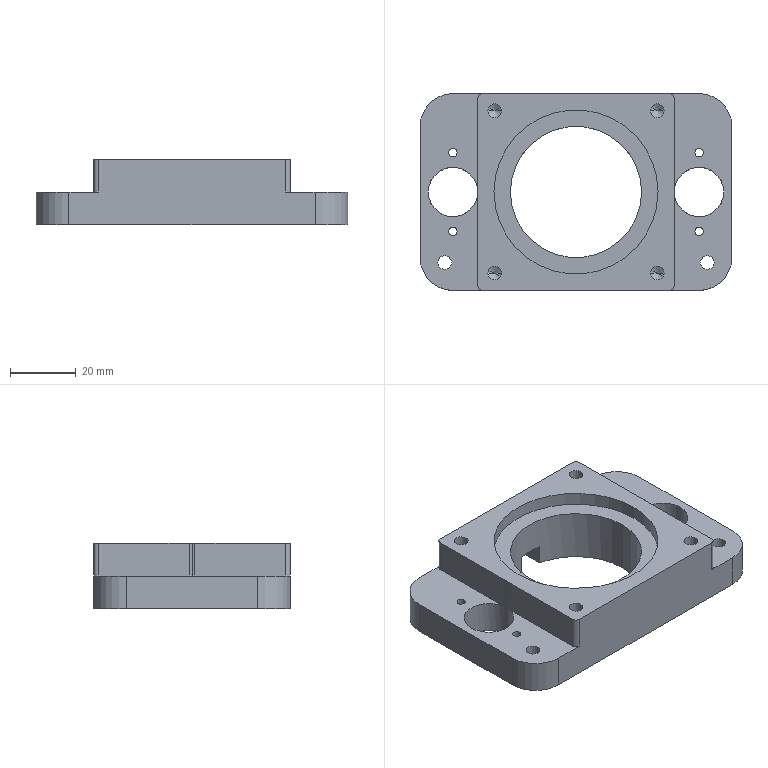Part | STEP file | 1 solid | 60 faces | box 95 x 60 x 20 mm | volume 58909 mm3 | cylinder 36 | plane 16 | cone 8 | commonest cylinder face diameters 4.2 x12 2.5 x8 3 x4 15.1 x4 20 x4 40 x2